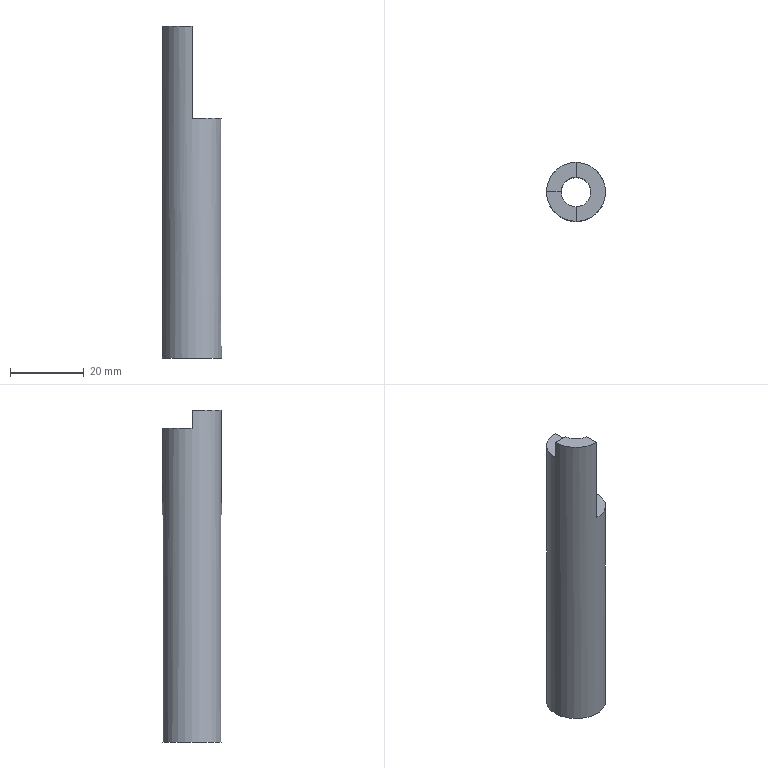Part | NX | features SWF 16-60 2 | 1 solid | 9 faces | box 16 x 16 x 90 mm | volume 11495 mm3 | plane 7 | cylinder 2 | commonest cylinder face diameters 8.003 x1 16 x1
STEP:
#1=CARTESIAN_POINT('',(2592.094,-780.621,830.716));
#2=VERTEX_POINT('',#1);
#3=CARTESIAN_POINT('',(2592.094,-776.622,830.716));
#4=VERTEX_POINT('',#3);
#5=CARTESIAN_POINT('',(2592.094,-980.056,830.716));
#6=DIRECTION('',(0.,1.,0.));
#7=VECTOR('',#6,1000.);
#8=LINE('',#5,#7);
#9=EDGE_CURVE('',#2,#4,#8,.T.);
#10=ORIENTED_EDGE('',*,*,#9,.F.);
#11=CARTESIAN_POINT('',(2592.094,-780.621,810.716));
#12=VERTEX_POINT('',#11);
#13=CARTESIAN_POINT('',(2592.094,-780.621,835.716));
#14=DIRECTION('',(0.,0.,-1.));
#15=VECTOR('',#14,1000.);
#16=LINE('',#13,#15);
#17=EDGE_CURVE('',#2,#12,#16,.T.);
#18=ORIENTED_EDGE('',*,*,#17,.T.);
#19=CARTESIAN_POINT('',(2592.094,-776.622,810.716));
#20=VERTEX_POINT('',#19);
#21=CARTESIAN_POINT('',(2592.094,-800.622,810.716));
#22=DIRECTION('',(0.,-1.,0.));
#23=VECTOR('',#22,1000.);
#24=LINE('',#21,#23);
#25=EDGE_CURVE('',#20,#12,#24,.T.);
#26=ORIENTED_EDGE('',*,*,#25,.F.);
#27=CARTESIAN_POINT('',(2592.094,-776.622,835.716));
#28=DIRECTION('',(0.,0.,-1.));
#29=VECTOR('',#28,1000.);
#30=LINE('',#27,#29);
#31=EDGE_CURVE('',#4,#20,#30,.T.);
#32=ORIENTED_EDGE('',*,*,#31,.F.);
#33=EDGE_LOOP('',(#10,#18,#26,#32));
#34=FACE_BOUND('',#33,.T.);
#35=CARTESIAN_POINT('',(2592.094,-800.622,813.716));
#36=DIRECTION('',(-1.,0.,0.));
#37=DIRECTION('',(0.,0.,-1.));
#38=AXIS2_PLACEMENT_3D('',#35,#36,#37);
#39=PLANE('',#38);
#40=ADVANCED_FACE('',(#34),#39,.F.);
#41=CARTESIAN_POINT('',(2596.095,-784.622,745.716));
#42=VERTEX_POINT('',#41);
#43=CARTESIAN_POINT('',(2592.094,-784.622,745.716));
#44=DIRECTION('',(0.,0.,-1.));
#45=DIRECTION('',(-1.,0.,0.));
#46=AXIS2_PLACEMENT_3D('',#43,#44,#45);
#47=CIRCLE('',#46,4.002);
#48=EDGE_CURVE('',#42,#42,#47,.T.);
#49=ORIENTED_EDGE('',*,*,#48,.F.);
#50=EDGE_LOOP('',(#49));
#51=FACE_BOUND('',#50,.T.);
#52=CARTESIAN_POINT('',(2600.094,-784.622,745.716));
#53=VERTEX_POINT('',#52);
#54=CARTESIAN_POINT('',(2592.094,-784.622,745.716));
#55=DIRECTION('',(0.,0.,-1.));
#56=DIRECTION('',(-1.,0.,0.));
#57=AXIS2_PLACEMENT_3D('',#54,#55,#56);
#58=CIRCLE('',#57,8.);
#59=EDGE_CURVE('',#53,#53,#58,.T.);
#60=ORIENTED_EDGE('',*,*,#59,.T.);
#61=EDGE_LOOP('',(#60));
#62=FACE_BOUND('',#61,.T.);
#63=CARTESIAN_POINT('',(2592.094,-784.622,745.716));
#64=DIRECTION('',(0.,0.,-1.));
#65=DIRECTION('',(1.,0.,0.));
#66=AXIS2_PLACEMENT_3D('',#63,#64,#65);
#67=PLANE('',#66);
#68=ADVANCED_FACE('',(#51,#62),#67,.T.);
#69=CARTESIAN_POINT('',(2588.092,-784.622,835.716));
#70=VERTEX_POINT('',#69);
#71=CARTESIAN_POINT('',(2584.094,-784.622,835.716));
#72=VERTEX_POINT('',#71);
#73=CARTESIAN_POINT('',(2592.094,-784.622,835.716));
#74=DIRECTION('',(-1.,0.,0.));
#75=VECTOR('',#74,1000.);
#76=LINE('',#73,#75);
#77=EDGE_CURVE('',#70,#72,#76,.T.);
#78=ORIENTED_EDGE('',*,*,#77,.T.);
#79=CARTESIAN_POINT('',(2592.094,-792.622,835.716));
#80=VERTEX_POINT('',#79);
#81=CARTESIAN_POINT('',(2592.094,-784.622,835.716));
#82=DIRECTION('',(0.,0.,1.));
#83=DIRECTION('',(1.,0.,0.));
#84=AXIS2_PLACEMENT_3D('',#81,#82,#83);
#85=CIRCLE('',#84,8.);
#86=EDGE_CURVE('',#72,#80,#85,.T.);
#87=ORIENTED_EDGE('',*,*,#86,.T.);
#88=CARTESIAN_POINT('',(2592.094,-788.624,835.716));
#89=VERTEX_POINT('',#88);
#90=CARTESIAN_POINT('',(2592.094,-800.622,835.716));
#91=DIRECTION('',(0.,1.,0.));
#92=VECTOR('',#91,1000.);
#93=LINE('',#90,#92);
#94=EDGE_CURVE('',#80,#89,#93,.T.);
#95=ORIENTED_EDGE('',*,*,#94,.T.);
#96=CARTESIAN_POINT('',(2592.094,-784.622,835.716));
#97=DIRECTION('',(0.,0.,1.));
#98=DIRECTION('',(1.,0.,0.));
#99=AXIS2_PLACEMENT_3D('',#96,#97,#98);
#100=CIRCLE('',#99,4.002);
#101=EDGE_CURVE('',#70,#89,#100,.T.);
#102=ORIENTED_EDGE('',*,*,#101,.F.);
#103=EDGE_LOOP('',(#78,#87,#95,#102));
#104=FACE_BOUND('',#103,.T.);
#105=CARTESIAN_POINT('',(2592.094,-784.622,835.716));
#106=DIRECTION('',(0.,0.,1.));
#107=DIRECTION('',(-1.,0.,0.));
#108=AXIS2_PLACEMENT_3D('',#105,#106,#107);
#109=PLANE('',#108);
#110=ADVANCED_FACE('',(#104),#109,.T.);
#111=CARTESIAN_POINT('',(2584.094,-784.622,830.716));
#112=VERTEX_POINT('',#111);
#113=CARTESIAN_POINT('',(2584.094,-784.622,835.716));
#114=DIRECTION('',(0.,0.,-1.));
#115=VECTOR('',#114,1000.);
#116=LINE('',#113,#115);
#117=EDGE_CURVE('',#72,#112,#116,.T.);
#118=ORIENTED_EDGE('',*,*,#117,.T.);
#119=CARTESIAN_POINT('',(2592.094,-784.622,830.716));
#120=DIRECTION('',(0.,0.,-1.));
#121=DIRECTION('',(1.,0.,0.));
#122=AXIS2_PLACEMENT_3D('',#119,#120,#121);
#123=CIRCLE('',#122,8.);
#124=EDGE_CURVE('',#4,#112,#123,.F.);
#125=ORIENTED_EDGE('',*,*,#124,.F.);
#126=ORIENTED_EDGE('',*,*,#31,.T.);
#127=CARTESIAN_POINT('',(2592.094,-792.622,810.716));
#128=VERTEX_POINT('',#127);
#129=CARTESIAN_POINT('',(2592.094,-784.622,810.716));
#130=DIRECTION('',(0.,0.,-1.));
#131=DIRECTION('',(-1.,0.,0.));
#132=AXIS2_PLACEMENT_3D('',#129,#130,#131);
#133=CIRCLE('',#132,8.);
#134=EDGE_CURVE('',#20,#128,#133,.T.);
#135=ORIENTED_EDGE('',*,*,#134,.T.);
#136=CARTESIAN_POINT('',(2592.094,-792.622,835.716));
#137=DIRECTION('',(0.,0.,1.));
#138=VECTOR('',#137,1000.);
#139=LINE('',#136,#138);
#140=EDGE_CURVE('',#128,#80,#139,.T.);
#141=ORIENTED_EDGE('',*,*,#140,.T.);
#142=ORIENTED_EDGE('',*,*,#86,.F.);
#143=EDGE_LOOP('',(#118,#125,#126,#135,#141,#142));
#144=FACE_BOUND('',#143,.T.);
#145=ORIENTED_EDGE('',*,*,#59,.F.);
#146=EDGE_LOOP('',(#145));
#147=FACE_BOUND('',#146,.T.);
#148=CARTESIAN_POINT('',(2592.094,-784.622,835.716));
#149=DIRECTION('',(0.,0.,-1.));
#150=DIRECTION('',(-1.,0.,0.));
#151=AXIS2_PLACEMENT_3D('',#148,#149,#150);
#152=CYLINDRICAL_SURFACE('',#151,8.);
#153=ADVANCED_FACE('',(#144,#147),#152,.T.);
#154=ORIENTED_EDGE('',*,*,#48,.T.);
#155=EDGE_LOOP('',(#154));
#156=FACE_BOUND('',#155,.T.);
#157=ORIENTED_EDGE('',*,*,#101,.T.);
#158=CARTESIAN_POINT('',(2592.094,-788.624,810.716));
#159=VERTEX_POINT('',#158);
#160=CARTESIAN_POINT('',(2592.094,-788.624,835.716));
#161=DIRECTION('',(0.,0.,1.));
#162=VECTOR('',#161,1000.);
#163=LINE('',#160,#162);
#164=EDGE_CURVE('',#159,#89,#163,.T.);
#165=ORIENTED_EDGE('',*,*,#164,.F.);
#166=CARTESIAN_POINT('',(2592.094,-784.622,810.716));
#167=DIRECTION('',(0.,0.,-1.));
#168=DIRECTION('',(-1.,0.,0.));
#169=AXIS2_PLACEMENT_3D('',#166,#167,#168);
#170=CIRCLE('',#169,4.002);
#171=EDGE_CURVE('',#12,#159,#170,.T.);
#172=ORIENTED_EDGE('',*,*,#171,.F.);
#173=ORIENTED_EDGE('',*,*,#17,.F.);
#174=CARTESIAN_POINT('',(2588.092,-784.622,830.716));
#175=VERTEX_POINT('',#174);
#176=CARTESIAN_POINT('',(2592.094,-784.622,830.716));
#177=DIRECTION('',(0.,0.,-1.));
#178=DIRECTION('',(1.,0.,0.));
#179=AXIS2_PLACEMENT_3D('',#176,#177,#178);
#180=CIRCLE('',#179,4.002);
#181=EDGE_CURVE('',#2,#175,#180,.F.);
#182=ORIENTED_EDGE('',*,*,#181,.T.);
#183=CARTESIAN_POINT('',(2588.092,-784.622,835.716));
#184=DIRECTION('',(0.,0.,-1.));
#185=VECTOR('',#184,1000.);
#186=LINE('',#183,#185);
#187=EDGE_CURVE('',#70,#175,#186,.T.);
#188=ORIENTED_EDGE('',*,*,#187,.F.);
#189=EDGE_LOOP('',(#157,#165,#172,#173,#182,#188));
#190=FACE_BOUND('',#189,.T.);
#191=CARTESIAN_POINT('',(2592.094,-784.622,835.716));
#192=DIRECTION('',(0.,0.,-1.));
#193=DIRECTION('',(-1.,0.,0.));
#194=AXIS2_PLACEMENT_3D('',#191,#192,#193);
#195=CYLINDRICAL_SURFACE('',#194,4.002);
#196=ADVANCED_FACE('',(#156,#190),#195,.F.);
#197=ORIENTED_EDGE('',*,*,#140,.F.);
#198=CARTESIAN_POINT('',(2592.094,-800.622,810.716));
#199=DIRECTION('',(0.,-1.,0.));
#200=VECTOR('',#199,1000.);
#201=LINE('',#198,#200);
#202=EDGE_CURVE('',#159,#128,#201,.T.);
#203=ORIENTED_EDGE('',*,*,#202,.F.);
#204=ORIENTED_EDGE('',*,*,#164,.T.);
#205=ORIENTED_EDGE('',*,*,#94,.F.);
#206=EDGE_LOOP('',(#197,#203,#204,#205));
#207=FACE_BOUND('',#206,.T.);
#208=CARTESIAN_POINT('',(2592.094,-800.622,813.716));
#209=DIRECTION('',(-1.,0.,0.));
#210=DIRECTION('',(0.,0.,-1.));
#211=AXIS2_PLACEMENT_3D('',#208,#209,#210);
#212=PLANE('',#211);
#213=ADVANCED_FACE('',(#207),#212,.F.);
#214=ORIENTED_EDGE('',*,*,#134,.F.);
#215=ORIENTED_EDGE('',*,*,#25,.T.);
#216=ORIENTED_EDGE('',*,*,#171,.T.);
#217=ORIENTED_EDGE('',*,*,#202,.T.);
#218=EDGE_LOOP('',(#214,#215,#216,#217));
#219=FACE_BOUND('',#218,.T.);
#220=CARTESIAN_POINT('',(2681.103,-980.056,810.716));
#221=DIRECTION('',(0.,0.,-1.));
#222=DIRECTION('',(1.,0.,0.));
#223=AXIS2_PLACEMENT_3D('',#220,#221,#222);
#224=PLANE('',#223);
#225=ADVANCED_FACE('',(#219),#224,.F.);
#226=ORIENTED_EDGE('',*,*,#117,.F.);
#227=ORIENTED_EDGE('',*,*,#77,.F.);
#228=ORIENTED_EDGE('',*,*,#187,.T.);
#229=CARTESIAN_POINT('',(2592.094,-784.622,830.716));
#230=DIRECTION('',(1.,0.,0.));
#231=VECTOR('',#230,1000.);
#232=LINE('',#229,#231);
#233=EDGE_CURVE('',#112,#175,#232,.T.);
#234=ORIENTED_EDGE('',*,*,#233,.F.);
#235=EDGE_LOOP('',(#226,#227,#228,#234));
#236=FACE_BOUND('',#235,.T.);
#237=CARTESIAN_POINT('',(2592.094,-784.622,833.716));
#238=DIRECTION('',(0.,-1.,0.));
#239=DIRECTION('',(0.,0.,-1.));
#240=AXIS2_PLACEMENT_3D('',#237,#238,#239);
#241=PLANE('',#240);
#242=ADVANCED_FACE('',(#236),#241,.F.);
#243=ORIENTED_EDGE('',*,*,#9,.T.);
#244=ORIENTED_EDGE('',*,*,#124,.T.);
#245=ORIENTED_EDGE('',*,*,#233,.T.);
#246=ORIENTED_EDGE('',*,*,#181,.F.);
#247=EDGE_LOOP('',(#243,#244,#245,#246));
#248=FACE_BOUND('',#247,.T.);
#249=CARTESIAN_POINT('',(2681.103,-980.056,830.716));
#250=DIRECTION('',(0.,0.,1.));
#251=DIRECTION('',(-1.,0.,0.));
#252=AXIS2_PLACEMENT_3D('',#249,#250,#251);
#253=PLANE('',#252);
#254=ADVANCED_FACE('',(#248),#253,.T.);
#255=CLOSED_SHELL('',(#40,#68,#110,#153,#196,#213,#225,#242,#254));
#256=MANIFOLD_SOLID_BREP('',#255);
#257=(LENGTH_UNIT()NAMED_UNIT(*)SI_UNIT(.MILLI.,.METRE.));
#258=UNCERTAINTY_MEASURE_WITH_UNIT(LENGTH_MEASURE(0.00001),#257,'','');
#259=(NAMED_UNIT(*)PLANE_ANGLE_UNIT()SI_UNIT($,.RADIAN.));
#260=(NAMED_UNIT(*)SI_UNIT($,.STERADIAN.)SOLID_ANGLE_UNIT());
#261=(GEOMETRIC_REPRESENTATION_CONTEXT(3)GLOBAL_UNCERTAINTY_ASSIGNED_CONTEXT((#258))GLOBAL_UNIT_ASSIGNED_CONTEXT((#257,#259,#260))REPRESENTATION_CONTEXT('',''));
#262=ADVANCED_BREP_SHAPE_REPRESENTATION('',(#256),#261);